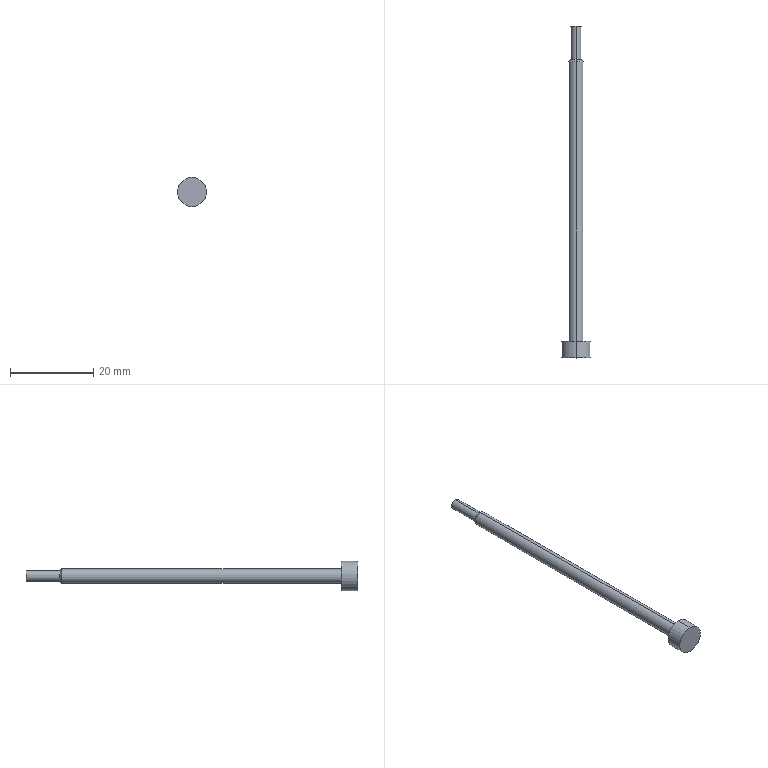Part | STEP file | 1 solid | 11 faces | box 7 x 79.697 x 7 mm | volume 843.527 mm3 | cylinder 6 | plane 3 | cone 2 | commonest cylinder face diameters 2.513 x2 3.5 x2 7 x2
STEP:
#1=CARTESIAN_POINT('',(0.,0.,0.));
#2=DIRECTION('',(0.,0.,1.));
#3=DIRECTION('',(1.,0.,0.));
#4=AXIS2_PLACEMENT_3D('',#1,#2,#3);
#5=CARTESIAN_POINT('',(-37.537,-40.,127.416));
#6=VERTEX_POINT('',#5);
#7=CARTESIAN_POINT('',(-37.537,-40.,120.416));
#8=VERTEX_POINT('',#7);
#9=CARTESIAN_POINT('',(-37.537,-40.,123.916));
#10=DIRECTION('',(0.,1.,0.));
#11=DIRECTION('',(0.,0.,-1.));
#12=AXIS2_PLACEMENT_3D('',#9,#10,#11);
#13=CIRCLE('',#12,3.5);
#14=CARTESIAN_POINT('',(-37.537,-50.,123.916));
#15=DIRECTION('',(0.,1.,0.));
#16=DIRECTION('',(0.,0.,1.));
#17=AXIS2_PLACEMENT_3D('',#14,#15,#16);
#18=CYLINDRICAL_SURFACE('',#17,3.5);
#19=CARTESIAN_POINT('',(-3.142,10.));
#20=DIRECTION('',(1.,0.));
#21=VECTOR('',#20,1.);
#22=LINE('',#19,#21);
#23=(GEOMETRIC_REPRESENTATION_CONTEXT(2)PARAMETRIC_REPRESENTATION_CONTEXT()REPRESENTATION_CONTEXT('',''));
#24=DEFINITIONAL_REPRESENTATION('',(#22),#23);
#25=PCURVE('',#18,#24);
#26=CARTESIAN_POINT('',(-72.862,-40.,23.556));
#27=DIRECTION('',(0.,-1.,0.));
#28=DIRECTION('',(0.,0.,-1.));
#29=AXIS2_PLACEMENT_3D('',#26,#27,#28);
#30=PLANE('',#29);
#31=CARTESIAN_POINT('',(-96.861,35.326));
#32=CARTESIAN_POINT('',(-96.861,29.264));
#33=CARTESIAN_POINT('',(-102.111,32.295));
#34=CARTESIAN_POINT('',(-107.361,35.326));
#35=CARTESIAN_POINT('',(-102.111,38.357));
#36=CARTESIAN_POINT('',(-96.861,41.388));
#37=CARTESIAN_POINT('',(-96.861,35.326));
#38=(BOUNDED_CURVE()B_SPLINE_CURVE(2,(#31,#32,#33,#34,#35,#36,#37),.UNSPECIFIED.,.T.,.F.)B_SPLINE_CURVE_WITH_KNOTS((1,2,2,2,2,1),(-2.094,0.,2.094,4.189,6.283,8.378),.UNSPECIFIED.)CURVE()GEOMETRIC_REPRESENTATION_ITEM()RATIONAL_B_SPLINE_CURVE((1.,0.5,1.,0.5,1.,0.5,1.))REPRESENTATION_ITEM(''));
#39=(GEOMETRIC_REPRESENTATION_CONTEXT(2)PARAMETRIC_REPRESENTATION_CONTEXT()REPRESENTATION_CONTEXT('',''));
#40=DEFINITIONAL_REPRESENTATION('',(#38),#39);
#41=PCURVE('',#30,#40);
#42=SURFACE_CURVE('',#13,(#25,#41),.PCURVE_S1.);
#43=EDGE_CURVE('',#6,#8,#42,.T.);
#44=ORIENTED_EDGE('',*,*,#43,.T.);
#45=CARTESIAN_POINT('',(-37.537,-36.,120.416));
#46=VERTEX_POINT('',#45);
#47=CARTESIAN_POINT('',(-37.537,-50.,120.416));
#48=DIRECTION('',(0.,1.,0.));
#49=VECTOR('',#48,1.);
#50=LINE('',#47,#49);
#51=CARTESIAN_POINT('',(3.142,0.));
#52=DIRECTION('',(0.,1.));
#53=VECTOR('',#52,1.);
#54=LINE('',#51,#53);
#55=(GEOMETRIC_REPRESENTATION_CONTEXT(2)PARAMETRIC_REPRESENTATION_CONTEXT()REPRESENTATION_CONTEXT('',''));
#56=DEFINITIONAL_REPRESENTATION('',(#54),#55);
#57=PCURVE('',#18,#56);
#58=CARTESIAN_POINT('',(-37.537,-50.,123.916));
#59=DIRECTION('',(0.,1.,0.));
#60=DIRECTION('',(0.,0.,1.));
#61=AXIS2_PLACEMENT_3D('',#58,#59,#60);
#62=CYLINDRICAL_SURFACE('',#61,3.5);
#63=CARTESIAN_POINT('',(3.142,0.));
#64=DIRECTION('',(0.,1.));
#65=VECTOR('',#64,1.);
#66=LINE('',#63,#65);
#67=(GEOMETRIC_REPRESENTATION_CONTEXT(2)PARAMETRIC_REPRESENTATION_CONTEXT()REPRESENTATION_CONTEXT('',''));
#68=DEFINITIONAL_REPRESENTATION('',(#66),#67);
#69=PCURVE('',#62,#68);
#70=SURFACE_CURVE('',#50,(#57,#69),.PCURVE_S1.);
#71=EDGE_CURVE('',#8,#46,#70,.T.);
#72=ORIENTED_EDGE('',*,*,#71,.T.);
#73=CARTESIAN_POINT('',(-37.537,-36.,127.416));
#74=VERTEX_POINT('',#73);
#75=CARTESIAN_POINT('',(-37.537,-36.,123.916));
#76=DIRECTION('',(0.,-1.,0.));
#77=DIRECTION('',(0.,0.,-1.));
#78=AXIS2_PLACEMENT_3D('',#75,#76,#77);
#79=CIRCLE('',#78,3.5);
#80=CARTESIAN_POINT('',(3.142,14.));
#81=DIRECTION('',(-1.,0.));
#82=VECTOR('',#81,1.);
#83=LINE('',#80,#82);
#84=(GEOMETRIC_REPRESENTATION_CONTEXT(2)PARAMETRIC_REPRESENTATION_CONTEXT()REPRESENTATION_CONTEXT('',''));
#85=DEFINITIONAL_REPRESENTATION('',(#83),#84);
#86=PCURVE('',#18,#85);
#87=CARTESIAN_POINT('',(-37.537,-36.,123.916));
#88=DIRECTION('',(0.,1.,0.));
#89=DIRECTION('',(0.,0.,1.));
#90=AXIS2_PLACEMENT_3D('',#87,#88,#89);
#91=PLANE('',#90);
#92=CARTESIAN_POINT('',(-3.5,0.));
#93=CARTESIAN_POINT('',(-3.5,6.062));
#94=CARTESIAN_POINT('',(1.75,3.031));
#95=CARTESIAN_POINT('',(7.,0.));
#96=CARTESIAN_POINT('',(1.75,-3.031));
#97=CARTESIAN_POINT('',(-3.5,-6.062));
#98=CARTESIAN_POINT('',(-3.5,0.));
#99=(BOUNDED_CURVE()B_SPLINE_CURVE(2,(#92,#93,#94,#95,#96,#97,#98),.UNSPECIFIED.,.T.,.F.)B_SPLINE_CURVE_WITH_KNOTS((1,2,2,2,2,1),(-2.094,0.,2.094,4.189,6.283,8.378),.UNSPECIFIED.)CURVE()GEOMETRIC_REPRESENTATION_ITEM()RATIONAL_B_SPLINE_CURVE((1.,0.5,1.,0.5,1.,0.5,1.))REPRESENTATION_ITEM(''));
#100=(GEOMETRIC_REPRESENTATION_CONTEXT(2)PARAMETRIC_REPRESENTATION_CONTEXT()REPRESENTATION_CONTEXT('',''));
#101=DEFINITIONAL_REPRESENTATION('',(#99),#100);
#102=PCURVE('',#91,#101);
#103=SURFACE_CURVE('',#79,(#86,#102),.PCURVE_S1.);
#104=EDGE_CURVE('',#46,#74,#103,.T.);
#105=ORIENTED_EDGE('',*,*,#104,.T.);
#106=CARTESIAN_POINT('',(-37.537,-50.,127.416));
#107=DIRECTION('',(0.,1.,0.));
#108=VECTOR('',#107,1.);
#109=LINE('',#106,#108);
#110=CARTESIAN_POINT('',(0.,0.));
#111=DIRECTION('',(0.,1.));
#112=VECTOR('',#111,1.);
#113=LINE('',#110,#112);
#114=(GEOMETRIC_REPRESENTATION_CONTEXT(2)PARAMETRIC_REPRESENTATION_CONTEXT()REPRESENTATION_CONTEXT('',''));
#115=DEFINITIONAL_REPRESENTATION('',(#113),#114);
#116=PCURVE('',#18,#115);
#117=CARTESIAN_POINT('',(6.283,0.));
#118=DIRECTION('',(0.,1.));
#119=VECTOR('',#118,1.);
#120=LINE('',#117,#119);
#121=(GEOMETRIC_REPRESENTATION_CONTEXT(2)PARAMETRIC_REPRESENTATION_CONTEXT()REPRESENTATION_CONTEXT('',''));
#122=DEFINITIONAL_REPRESENTATION('',(#120),#121);
#123=PCURVE('',#62,#122);
#124=SURFACE_CURVE('',#109,(#116,#123),.PCURVE_S1.);
#125=EDGE_CURVE('',#6,#74,#124,.T.);
#126=ORIENTED_EDGE('',*,*,#125,.F.);
#127=EDGE_LOOP('',(#44,#72,#105,#126));
#128=FACE_BOUND('',#127,.T.);
#129=ADVANCED_FACE('',(#128),#18,.T.);
#130=CARTESIAN_POINT('',(-37.537,31.164,125.666));
#131=VERTEX_POINT('',#130);
#132=CARTESIAN_POINT('',(-37.537,31.164,122.166));
#133=VERTEX_POINT('',#132);
#134=CARTESIAN_POINT('',(-37.537,31.164,123.916));
#135=DIRECTION('',(0.,1.,0.));
#136=DIRECTION('',(0.,0.,-1.));
#137=AXIS2_PLACEMENT_3D('',#134,#135,#136);
#138=CIRCLE('',#137,1.75);
#139=CARTESIAN_POINT('',(-37.537,39.697,123.916));
#140=DIRECTION('',(0.,-1.,0.));
#141=DIRECTION('',(0.,0.,-1.));
#142=AXIS2_PLACEMENT_3D('',#139,#140,#141);
#143=CYLINDRICAL_SURFACE('',#142,1.75);
#144=CARTESIAN_POINT('',(6.283,8.534));
#145=DIRECTION('',(-1.,0.));
#146=VECTOR('',#145,1.);
#147=LINE('',#144,#146);
#148=(GEOMETRIC_REPRESENTATION_CONTEXT(2)PARAMETRIC_REPRESENTATION_CONTEXT()REPRESENTATION_CONTEXT('',''));
#149=DEFINITIONAL_REPRESENTATION('',(#147),#148);
#150=PCURVE('',#143,#149);
#151=CARTESIAN_POINT('',(-37.537,31.657,123.916));
#152=DIRECTION('',(0.,-1.,0.));
#153=DIRECTION('',(0.,0.,-1.));
#154=AXIS2_PLACEMENT_3D('',#151,#152,#153);
#155=CONICAL_SURFACE('',#154,1.256,0.7854);
#156=CARTESIAN_POINT('',(6.283,0.4938));
#157=DIRECTION('',(-1.,0.));
#158=VECTOR('',#157,1.);
#159=LINE('',#156,#158);
#160=(GEOMETRIC_REPRESENTATION_CONTEXT(2)PARAMETRIC_REPRESENTATION_CONTEXT()REPRESENTATION_CONTEXT('',''));
#161=DEFINITIONAL_REPRESENTATION('',(#159),#160);
#162=PCURVE('',#155,#161);
#163=SURFACE_CURVE('',#138,(#150,#162),.PCURVE_S1.);
#164=EDGE_CURVE('',#131,#133,#163,.T.);
#165=ORIENTED_EDGE('',*,*,#164,.F.);
#166=CARTESIAN_POINT('',(-37.537,-36.,125.666));
#167=VERTEX_POINT('',#166);
#168=CARTESIAN_POINT('',(-37.537,39.697,125.666));
#169=DIRECTION('',(0.,-1.,0.));
#170=VECTOR('',#169,1.);
#171=LINE('',#168,#170);
#172=CARTESIAN_POINT('',(3.142,0.));
#173=DIRECTION('',(0.,1.));
#174=VECTOR('',#173,1.);
#175=LINE('',#172,#174);
#176=(GEOMETRIC_REPRESENTATION_CONTEXT(2)PARAMETRIC_REPRESENTATION_CONTEXT()REPRESENTATION_CONTEXT('',''));
#177=DEFINITIONAL_REPRESENTATION('',(#175),#176);
#178=PCURVE('',#143,#177);
#179=CARTESIAN_POINT('',(-37.537,39.697,123.916));
#180=DIRECTION('',(0.,-1.,0.));
#181=DIRECTION('',(0.,0.,-1.));
#182=AXIS2_PLACEMENT_3D('',#179,#180,#181);
#183=CYLINDRICAL_SURFACE('',#182,1.75);
#184=CARTESIAN_POINT('',(3.142,0.));
#185=DIRECTION('',(0.,1.));
#186=VECTOR('',#185,1.);
#187=LINE('',#184,#186);
#188=(GEOMETRIC_REPRESENTATION_CONTEXT(2)PARAMETRIC_REPRESENTATION_CONTEXT()REPRESENTATION_CONTEXT('',''));
#189=DEFINITIONAL_REPRESENTATION('',(#187),#188);
#190=PCURVE('',#183,#189);
#191=SURFACE_CURVE('',#171,(#178,#190),.PCURVE_S1.);
#192=EDGE_CURVE('',#131,#167,#191,.T.);
#193=ORIENTED_EDGE('',*,*,#192,.T.);
#194=CARTESIAN_POINT('',(-37.537,-36.,122.166));
#195=VERTEX_POINT('',#194);
#196=CARTESIAN_POINT('',(-37.537,-36.,123.916));
#197=DIRECTION('',(0.,-1.,0.));
#198=DIRECTION('',(0.,0.,1.));
#199=AXIS2_PLACEMENT_3D('',#196,#197,#198);
#200=CIRCLE('',#199,1.75);
#201=CARTESIAN_POINT('',(-3.142,75.698));
#202=DIRECTION('',(1.,0.));
#203=VECTOR('',#202,1.);
#204=LINE('',#201,#203);
#205=(GEOMETRIC_REPRESENTATION_CONTEXT(2)PARAMETRIC_REPRESENTATION_CONTEXT()REPRESENTATION_CONTEXT('',''));
#206=DEFINITIONAL_REPRESENTATION('',(#204),#205);
#207=PCURVE('',#143,#206);
#208=CARTESIAN_POINT('',(1.75,0.));
#209=CARTESIAN_POINT('',(1.75,-3.031));
#210=CARTESIAN_POINT('',(-0.875,-1.516));
#211=CARTESIAN_POINT('',(-3.5,0.));
#212=CARTESIAN_POINT('',(-0.875,1.516));
#213=CARTESIAN_POINT('',(1.75,3.031));
#214=CARTESIAN_POINT('',(1.75,0.));
#215=(BOUNDED_CURVE()B_SPLINE_CURVE(2,(#208,#209,#210,#211,#212,#213,#214),.UNSPECIFIED.,.T.,.F.)B_SPLINE_CURVE_WITH_KNOTS((1,2,2,2,2,1),(-2.094,0.,2.094,4.189,6.283,8.378),.UNSPECIFIED.)CURVE()GEOMETRIC_REPRESENTATION_ITEM()RATIONAL_B_SPLINE_CURVE((1.,0.5,1.,0.5,1.,0.5,1.))REPRESENTATION_ITEM(''));
#216=(GEOMETRIC_REPRESENTATION_CONTEXT(2)PARAMETRIC_REPRESENTATION_CONTEXT()REPRESENTATION_CONTEXT('',''));
#217=DEFINITIONAL_REPRESENTATION('',(#215),#216);
#218=PCURVE('',#91,#217);
#219=SURFACE_CURVE('',#200,(#207,#218),.PCURVE_S1.);
#220=EDGE_CURVE('',#195,#167,#219,.T.);
#221=ORIENTED_EDGE('',*,*,#220,.F.);
#222=CARTESIAN_POINT('',(-37.537,39.697,122.166));
#223=DIRECTION('',(0.,-1.,0.));
#224=VECTOR('',#223,1.);
#225=LINE('',#222,#224);
#226=CARTESIAN_POINT('',(0.,0.));
#227=DIRECTION('',(0.,1.));
#228=VECTOR('',#227,1.);
#229=LINE('',#226,#228);
#230=(GEOMETRIC_REPRESENTATION_CONTEXT(2)PARAMETRIC_REPRESENTATION_CONTEXT()REPRESENTATION_CONTEXT('',''));
#231=DEFINITIONAL_REPRESENTATION('',(#229),#230);
#232=PCURVE('',#143,#231);
#233=CARTESIAN_POINT('',(6.283,0.));
#234=DIRECTION('',(0.,1.));
#235=VECTOR('',#234,1.);
#236=LINE('',#233,#235);
#237=(GEOMETRIC_REPRESENTATION_CONTEXT(2)PARAMETRIC_REPRESENTATION_CONTEXT()REPRESENTATION_CONTEXT('',''));
#238=DEFINITIONAL_REPRESENTATION('',(#236),#237);
#239=PCURVE('',#183,#238);
#240=SURFACE_CURVE('',#225,(#232,#239),.PCURVE_S1.);
#241=EDGE_CURVE('',#133,#195,#240,.T.);
#242=ORIENTED_EDGE('',*,*,#241,.F.);
#243=EDGE_LOOP('',(#165,#193,#221,#242));
#244=FACE_BOUND('',#243,.T.);
#245=ADVANCED_FACE('',(#244),#143,.T.);
#246=CARTESIAN_POINT('',(-37.537,31.657,122.66));
#247=VERTEX_POINT('',#246);
#248=CARTESIAN_POINT('',(-37.537,31.657,125.173));
#249=VERTEX_POINT('',#248);
#250=CARTESIAN_POINT('',(-37.537,31.657,123.916));
#251=DIRECTION('',(0.,-1.,0.));
#252=DIRECTION('',(0.,0.,-1.));
#253=AXIS2_PLACEMENT_3D('',#250,#251,#252);
#254=CIRCLE('',#253,1.256);
#255=CARTESIAN_POINT('',(0.,0.));
#256=DIRECTION('',(1.,0.));
#257=VECTOR('',#256,1.);
#258=LINE('',#255,#257);
#259=(GEOMETRIC_REPRESENTATION_CONTEXT(2)PARAMETRIC_REPRESENTATION_CONTEXT()REPRESENTATION_CONTEXT('',''));
#260=DEFINITIONAL_REPRESENTATION('',(#258),#259);
#261=PCURVE('',#155,#260);
#262=CARTESIAN_POINT('',(-37.537,39.697,123.916));
#263=DIRECTION('',(0.,-1.,0.));
#264=DIRECTION('',(0.,0.,-1.));
#265=AXIS2_PLACEMENT_3D('',#262,#263,#264);
#266=CYLINDRICAL_SURFACE('',#265,1.256);
#267=CARTESIAN_POINT('',(0.,8.04));
#268=DIRECTION('',(1.,0.));
#269=VECTOR('',#268,1.);
#270=LINE('',#267,#269);
#271=(GEOMETRIC_REPRESENTATION_CONTEXT(2)PARAMETRIC_REPRESENTATION_CONTEXT()REPRESENTATION_CONTEXT('',''));
#272=DEFINITIONAL_REPRESENTATION('',(#270),#271);
#273=PCURVE('',#266,#272);
#274=SURFACE_CURVE('',#254,(#261,#273),.PCURVE_S1.);
#275=EDGE_CURVE('',#247,#249,#274,.T.);
#276=ORIENTED_EDGE('',*,*,#275,.T.);
#277=CARTESIAN_POINT('',(-37.537,31.657,125.173));
#278=DIRECTION('',(0.,-0.7071,0.7071));
#279=VECTOR('',#278,1.);
#280=LINE('',#277,#279);
#281=CARTESIAN_POINT('',(3.142,0.));
#282=DIRECTION('',(0.,1.));
#283=VECTOR('',#282,1.);
#284=LINE('',#281,#283);
#285=(GEOMETRIC_REPRESENTATION_CONTEXT(2)PARAMETRIC_REPRESENTATION_CONTEXT()REPRESENTATION_CONTEXT('',''));
#286=DEFINITIONAL_REPRESENTATION('',(#284),#285);
#287=PCURVE('',#155,#286);
#288=CARTESIAN_POINT('',(-37.537,31.657,123.916));
#289=DIRECTION('',(0.,-1.,0.));
#290=DIRECTION('',(0.,0.,-1.));
#291=AXIS2_PLACEMENT_3D('',#288,#289,#290);
#292=CONICAL_SURFACE('',#291,1.256,0.7854);
#293=CARTESIAN_POINT('',(3.142,0.));
#294=DIRECTION('',(0.,1.));
#295=VECTOR('',#294,1.);
#296=LINE('',#293,#295);
#297=(GEOMETRIC_REPRESENTATION_CONTEXT(2)PARAMETRIC_REPRESENTATION_CONTEXT()REPRESENTATION_CONTEXT('',''));
#298=DEFINITIONAL_REPRESENTATION('',(#296),#297);
#299=PCURVE('',#292,#298);
#300=SURFACE_CURVE('',#280,(#287,#299),.PCURVE_S1.);
#301=EDGE_CURVE('',#249,#131,#300,.T.);
#302=ORIENTED_EDGE('',*,*,#301,.T.);
#303=ORIENTED_EDGE('',*,*,#164,.T.);
#304=CARTESIAN_POINT('',(-37.537,31.657,122.66));
#305=DIRECTION('',(0.,-0.7071,-0.7071));
#306=VECTOR('',#305,1.);
#307=LINE('',#304,#306);
#308=CARTESIAN_POINT('',(0.,0.));
#309=DIRECTION('',(0.,1.));
#310=VECTOR('',#309,1.);
#311=LINE('',#308,#310);
#312=(GEOMETRIC_REPRESENTATION_CONTEXT(2)PARAMETRIC_REPRESENTATION_CONTEXT()REPRESENTATION_CONTEXT('',''));
#313=DEFINITIONAL_REPRESENTATION('',(#311),#312);
#314=PCURVE('',#155,#313);
#315=CARTESIAN_POINT('',(6.283,0.));
#316=DIRECTION('',(0.,1.));
#317=VECTOR('',#316,1.);
#318=LINE('',#315,#317);
#319=(GEOMETRIC_REPRESENTATION_CONTEXT(2)PARAMETRIC_REPRESENTATION_CONTEXT()REPRESENTATION_CONTEXT('',''));
#320=DEFINITIONAL_REPRESENTATION('',(#318),#319);
#321=PCURVE('',#292,#320);
#322=SURFACE_CURVE('',#307,(#314,#321),.PCURVE_S1.);
#323=EDGE_CURVE('',#247,#133,#322,.T.);
#324=ORIENTED_EDGE('',*,*,#323,.F.);
#325=EDGE_LOOP('',(#276,#302,#303,#324));
#326=FACE_BOUND('',#325,.T.);
#327=ADVANCED_FACE('',(#326),#155,.T.);
#328=CARTESIAN_POINT('',(-37.537,39.697,122.66));
#329=VERTEX_POINT('',#328);
#330=CARTESIAN_POINT('',(-37.537,39.697,125.173));
#331=VERTEX_POINT('',#330);
#332=CARTESIAN_POINT('',(-37.537,39.697,123.916));
#333=DIRECTION('',(0.,-1.,0.));
#334=DIRECTION('',(0.,0.,-1.));
#335=AXIS2_PLACEMENT_3D('',#332,#333,#334);
#336=CIRCLE('',#335,1.256);
#337=CARTESIAN_POINT('',(0.,0.));
#338=DIRECTION('',(1.,0.));
#339=VECTOR('',#338,1.);
#340=LINE('',#337,#339);
#341=(GEOMETRIC_REPRESENTATION_CONTEXT(2)PARAMETRIC_REPRESENTATION_CONTEXT()REPRESENTATION_CONTEXT('',''));
#342=DEFINITIONAL_REPRESENTATION('',(#340),#341);
#343=PCURVE('',#266,#342);
#344=CARTESIAN_POINT('',(-37.537,39.697,123.916));
#345=DIRECTION('',(0.,1.,0.));
#346=DIRECTION('',(0.,0.,1.));
#347=AXIS2_PLACEMENT_3D('',#344,#345,#346);
#348=PLANE('',#347);
#349=CARTESIAN_POINT('',(-1.256,0.));
#350=CARTESIAN_POINT('',(-1.256,2.176));
#351=CARTESIAN_POINT('',(0.6281,1.088));
#352=CARTESIAN_POINT('',(2.513,0.));
#353=CARTESIAN_POINT('',(0.6281,-1.088));
#354=CARTESIAN_POINT('',(-1.256,-2.176));
#355=CARTESIAN_POINT('',(-1.256,0.));
#356=(BOUNDED_CURVE()B_SPLINE_CURVE(2,(#349,#350,#351,#352,#353,#354,#355),.UNSPECIFIED.,.T.,.F.)B_SPLINE_CURVE_WITH_KNOTS((1,2,2,2,2,1),(-2.094,0.,2.094,4.189,6.283,8.378),.UNSPECIFIED.)CURVE()GEOMETRIC_REPRESENTATION_ITEM()RATIONAL_B_SPLINE_CURVE((1.,0.5,1.,0.5,1.,0.5,1.))REPRESENTATION_ITEM(''));
#357=(GEOMETRIC_REPRESENTATION_CONTEXT(2)PARAMETRIC_REPRESENTATION_CONTEXT()REPRESENTATION_CONTEXT('',''));
#358=DEFINITIONAL_REPRESENTATION('',(#356),#357);
#359=PCURVE('',#348,#358);
#360=SURFACE_CURVE('',#336,(#343,#359),.PCURVE_S1.);
#361=EDGE_CURVE('',#329,#331,#360,.T.);
#362=ORIENTED_EDGE('',*,*,#361,.T.);
#363=CARTESIAN_POINT('',(-37.537,39.697,125.173));
#364=DIRECTION('',(0.,-1.,0.));
#365=VECTOR('',#364,1.);
#366=LINE('',#363,#365);
#367=CARTESIAN_POINT('',(3.142,0.));
#368=DIRECTION('',(0.,1.));
#369=VECTOR('',#368,1.);
#370=LINE('',#367,#369);
#371=(GEOMETRIC_REPRESENTATION_CONTEXT(2)PARAMETRIC_REPRESENTATION_CONTEXT()REPRESENTATION_CONTEXT('',''));
#372=DEFINITIONAL_REPRESENTATION('',(#370),#371);
#373=PCURVE('',#266,#372);
#374=CARTESIAN_POINT('',(-37.537,39.697,123.916));
#375=DIRECTION('',(0.,-1.,0.));
#376=DIRECTION('',(0.,0.,-1.));
#377=AXIS2_PLACEMENT_3D('',#374,#375,#376);
#378=CYLINDRICAL_SURFACE('',#377,1.256);
#379=CARTESIAN_POINT('',(3.142,0.));
#380=DIRECTION('',(0.,1.));
#381=VECTOR('',#380,1.);
#382=LINE('',#379,#381);
#383=(GEOMETRIC_REPRESENTATION_CONTEXT(2)PARAMETRIC_REPRESENTATION_CONTEXT()REPRESENTATION_CONTEXT('',''));
#384=DEFINITIONAL_REPRESENTATION('',(#382),#383);
#385=PCURVE('',#378,#384);
#386=SURFACE_CURVE('',#366,(#373,#385),.PCURVE_S1.);
#387=EDGE_CURVE('',#331,#249,#386,.T.);
#388=ORIENTED_EDGE('',*,*,#387,.T.);
#389=ORIENTED_EDGE('',*,*,#275,.F.);
#390=CARTESIAN_POINT('',(-37.537,39.697,122.66));
#391=DIRECTION('',(0.,-1.,0.));
#392=VECTOR('',#391,1.);
#393=LINE('',#390,#392);
#394=CARTESIAN_POINT('',(0.,0.));
#395=DIRECTION('',(0.,1.));
#396=VECTOR('',#395,1.);
#397=LINE('',#394,#396);
#398=(GEOMETRIC_REPRESENTATION_CONTEXT(2)PARAMETRIC_REPRESENTATION_CONTEXT()REPRESENTATION_CONTEXT('',''));
#399=DEFINITIONAL_REPRESENTATION('',(#397),#398);
#400=PCURVE('',#266,#399);
#401=CARTESIAN_POINT('',(6.283,0.));
#402=DIRECTION('',(0.,1.));
#403=VECTOR('',#402,1.);
#404=LINE('',#401,#403);
#405=(GEOMETRIC_REPRESENTATION_CONTEXT(2)PARAMETRIC_REPRESENTATION_CONTEXT()REPRESENTATION_CONTEXT('',''));
#406=DEFINITIONAL_REPRESENTATION('',(#404),#405);
#407=PCURVE('',#378,#406);
#408=SURFACE_CURVE('',#393,(#400,#407),.PCURVE_S1.);
#409=EDGE_CURVE('',#329,#247,#408,.T.);
#410=ORIENTED_EDGE('',*,*,#409,.F.);
#411=EDGE_LOOP('',(#362,#388,#389,#410));
#412=FACE_BOUND('',#411,.T.);
#413=ADVANCED_FACE('',(#412),#266,.T.);
#414=ORIENTED_EDGE('',*,*,#387,.F.);
#415=CARTESIAN_POINT('',(-37.537,39.697,123.916));
#416=DIRECTION('',(0.,-1.,0.));
#417=DIRECTION('',(0.,0.,-1.));
#418=AXIS2_PLACEMENT_3D('',#415,#416,#417);
#419=CIRCLE('',#418,1.256);
#420=CARTESIAN_POINT('',(0.,0.));
#421=DIRECTION('',(1.,0.));
#422=VECTOR('',#421,1.);
#423=LINE('',#420,#422);
#424=(GEOMETRIC_REPRESENTATION_CONTEXT(2)PARAMETRIC_REPRESENTATION_CONTEXT()REPRESENTATION_CONTEXT('',''));
#425=DEFINITIONAL_REPRESENTATION('',(#423),#424);
#426=PCURVE('',#378,#425);
#427=CARTESIAN_POINT('',(-1.256,0.));
#428=CARTESIAN_POINT('',(-1.256,2.176));
#429=CARTESIAN_POINT('',(0.6281,1.088));
#430=CARTESIAN_POINT('',(2.513,0.));
#431=CARTESIAN_POINT('',(0.6281,-1.088));
#432=CARTESIAN_POINT('',(-1.256,-2.176));
#433=CARTESIAN_POINT('',(-1.256,0.));
#434=(BOUNDED_CURVE()B_SPLINE_CURVE(2,(#427,#428,#429,#430,#431,#432,#433),.UNSPECIFIED.,.T.,.F.)B_SPLINE_CURVE_WITH_KNOTS((1,2,2,2,2,1),(-2.094,0.,2.094,4.189,6.283,8.378),.UNSPECIFIED.)CURVE()GEOMETRIC_REPRESENTATION_ITEM()RATIONAL_B_SPLINE_CURVE((1.,0.5,1.,0.5,1.,0.5,1.))REPRESENTATION_ITEM(''));
#435=(GEOMETRIC_REPRESENTATION_CONTEXT(2)PARAMETRIC_REPRESENTATION_CONTEXT()REPRESENTATION_CONTEXT('',''));
#436=DEFINITIONAL_REPRESENTATION('',(#434),#435);
#437=PCURVE('',#348,#436);
#438=SURFACE_CURVE('',#419,(#426,#437),.PCURVE_S1.);
#439=EDGE_CURVE('',#331,#329,#438,.T.);
#440=ORIENTED_EDGE('',*,*,#439,.T.);
#441=ORIENTED_EDGE('',*,*,#409,.T.);
#442=CARTESIAN_POINT('',(-37.537,31.657,123.916));
#443=DIRECTION('',(0.,-1.,0.));
#444=DIRECTION('',(0.,0.,-1.));
#445=AXIS2_PLACEMENT_3D('',#442,#443,#444);
#446=CIRCLE('',#445,1.256);
#447=CARTESIAN_POINT('',(0.,8.04));
#448=DIRECTION('',(1.,0.));
#449=VECTOR('',#448,1.);
#450=LINE('',#447,#449);
#451=(GEOMETRIC_REPRESENTATION_CONTEXT(2)PARAMETRIC_REPRESENTATION_CONTEXT()REPRESENTATION_CONTEXT('',''));
#452=DEFINITIONAL_REPRESENTATION('',(#450),#451);
#453=PCURVE('',#378,#452);
#454=CARTESIAN_POINT('',(0.,0.));
#455=DIRECTION('',(1.,0.));
#456=VECTOR('',#455,1.);
#457=LINE('',#454,#456);
#458=(GEOMETRIC_REPRESENTATION_CONTEXT(2)PARAMETRIC_REPRESENTATION_CONTEXT()REPRESENTATION_CONTEXT('',''));
#459=DEFINITIONAL_REPRESENTATION('',(#457),#458);
#460=PCURVE('',#292,#459);
#461=SURFACE_CURVE('',#446,(#453,#460),.PCURVE_S1.);
#462=EDGE_CURVE('',#249,#247,#461,.T.);
#463=ORIENTED_EDGE('',*,*,#462,.F.);
#464=EDGE_LOOP('',(#414,#440,#441,#463));
#465=FACE_BOUND('',#464,.T.);
#466=ADVANCED_FACE('',(#465),#378,.T.);
#467=ORIENTED_EDGE('',*,*,#301,.F.);
#468=ORIENTED_EDGE('',*,*,#462,.T.);
#469=ORIENTED_EDGE('',*,*,#323,.T.);
#470=CARTESIAN_POINT('',(-37.537,31.164,123.916));
#471=DIRECTION('',(0.,1.,0.));
#472=DIRECTION('',(0.,0.,-1.));
#473=AXIS2_PLACEMENT_3D('',#470,#471,#472);
#474=CIRCLE('',#473,1.75);
#475=CARTESIAN_POINT('',(6.283,0.4938));
#476=DIRECTION('',(-1.,0.));
#477=VECTOR('',#476,1.);
#478=LINE('',#475,#477);
#479=(GEOMETRIC_REPRESENTATION_CONTEXT(2)PARAMETRIC_REPRESENTATION_CONTEXT()REPRESENTATION_CONTEXT('',''));
#480=DEFINITIONAL_REPRESENTATION('',(#478),#479);
#481=PCURVE('',#292,#480);
#482=CARTESIAN_POINT('',(6.283,8.534));
#483=DIRECTION('',(-1.,0.));
#484=VECTOR('',#483,1.);
#485=LINE('',#482,#484);
#486=(GEOMETRIC_REPRESENTATION_CONTEXT(2)PARAMETRIC_REPRESENTATION_CONTEXT()REPRESENTATION_CONTEXT('',''));
#487=DEFINITIONAL_REPRESENTATION('',(#485),#486);
#488=PCURVE('',#183,#487);
#489=SURFACE_CURVE('',#474,(#481,#488),.PCURVE_S1.);
#490=EDGE_CURVE('',#133,#131,#489,.T.);
#491=ORIENTED_EDGE('',*,*,#490,.T.);
#492=EDGE_LOOP('',(#467,#468,#469,#491));
#493=FACE_BOUND('',#492,.T.);
#494=ADVANCED_FACE('',(#493),#292,.T.);
#495=ORIENTED_EDGE('',*,*,#192,.F.);
#496=ORIENTED_EDGE('',*,*,#490,.F.);
#497=ORIENTED_EDGE('',*,*,#241,.T.);
#498=CARTESIAN_POINT('',(-37.537,-36.,123.916));
#499=DIRECTION('',(0.,-1.,0.));
#500=DIRECTION('',(0.,0.,1.));
#501=AXIS2_PLACEMENT_3D('',#498,#499,#500);
#502=CIRCLE('',#501,1.75);
#503=CARTESIAN_POINT('',(3.142,75.698));
#504=DIRECTION('',(1.,0.));
#505=VECTOR('',#504,1.);
#506=LINE('',#503,#505);
#507=(GEOMETRIC_REPRESENTATION_CONTEXT(2)PARAMETRIC_REPRESENTATION_CONTEXT()REPRESENTATION_CONTEXT('',''));
#508=DEFINITIONAL_REPRESENTATION('',(#506),#507);
#509=PCURVE('',#183,#508);
#510=CARTESIAN_POINT('',(1.75,0.));
#511=CARTESIAN_POINT('',(1.75,-3.031));
#512=CARTESIAN_POINT('',(-0.875,-1.516));
#513=CARTESIAN_POINT('',(-3.5,0.));
#514=CARTESIAN_POINT('',(-0.875,1.516));
#515=CARTESIAN_POINT('',(1.75,3.031));
#516=CARTESIAN_POINT('',(1.75,0.));
#517=(BOUNDED_CURVE()B_SPLINE_CURVE(2,(#510,#511,#512,#513,#514,#515,#516),.UNSPECIFIED.,.T.,.F.)B_SPLINE_CURVE_WITH_KNOTS((1,2,2,2,2,1),(-2.094,0.,2.094,4.189,6.283,8.378),.UNSPECIFIED.)CURVE()GEOMETRIC_REPRESENTATION_ITEM()RATIONAL_B_SPLINE_CURVE((1.,0.5,1.,0.5,1.,0.5,1.))REPRESENTATION_ITEM(''));
#518=(GEOMETRIC_REPRESENTATION_CONTEXT(2)PARAMETRIC_REPRESENTATION_CONTEXT()REPRESENTATION_CONTEXT('',''));
#519=DEFINITIONAL_REPRESENTATION('',(#517),#518);
#520=PCURVE('',#91,#519);
#521=SURFACE_CURVE('',#502,(#509,#520),.PCURVE_S1.);
#522=EDGE_CURVE('',#167,#195,#521,.T.);
#523=ORIENTED_EDGE('',*,*,#522,.F.);
#524=EDGE_LOOP('',(#495,#496,#497,#523));
#525=FACE_BOUND('',#524,.T.);
#526=ADVANCED_FACE('',(#525),#183,.T.);
#527=ORIENTED_EDGE('',*,*,#361,.F.);
#528=ORIENTED_EDGE('',*,*,#439,.F.);
#529=EDGE_LOOP('',(#527,#528));
#530=FACE_BOUND('',#529,.T.);
#531=ADVANCED_FACE('',(#530),#348,.T.);
#532=ORIENTED_EDGE('',*,*,#220,.T.);
#533=ORIENTED_EDGE('',*,*,#522,.T.);
#534=EDGE_LOOP('',(#532,#533));
#535=FACE_BOUND('',#534,.T.);
#536=CARTESIAN_POINT('',(-37.537,-36.,123.916));
#537=DIRECTION('',(0.,-1.,0.));
#538=DIRECTION('',(0.,0.,-1.));
#539=AXIS2_PLACEMENT_3D('',#536,#537,#538);
#540=CIRCLE('',#539,3.5);
#541=CARTESIAN_POINT('',(-3.5,0.));
#542=CARTESIAN_POINT('',(-3.5,6.062));
#543=CARTESIAN_POINT('',(1.75,3.031));
#544=CARTESIAN_POINT('',(7.,0.));
#545=CARTESIAN_POINT('',(1.75,-3.031));
#546=CARTESIAN_POINT('',(-3.5,-6.062));
#547=CARTESIAN_POINT('',(-3.5,0.));
#548=(BOUNDED_CURVE()B_SPLINE_CURVE(2,(#541,#542,#543,#544,#545,#546,#547),.UNSPECIFIED.,.T.,.F.)B_SPLINE_CURVE_WITH_KNOTS((1,2,2,2,2,1),(-2.094,0.,2.094,4.189,6.283,8.378),.UNSPECIFIED.)CURVE()GEOMETRIC_REPRESENTATION_ITEM()RATIONAL_B_SPLINE_CURVE((1.,0.5,1.,0.5,1.,0.5,1.))REPRESENTATION_ITEM(''));
#549=(GEOMETRIC_REPRESENTATION_CONTEXT(2)PARAMETRIC_REPRESENTATION_CONTEXT()REPRESENTATION_CONTEXT('',''));
#550=DEFINITIONAL_REPRESENTATION('',(#548),#549);
#551=PCURVE('',#91,#550);
#552=CARTESIAN_POINT('',(9.425,14.));
#553=DIRECTION('',(-1.,0.));
#554=VECTOR('',#553,1.);
#555=LINE('',#552,#554);
#556=(GEOMETRIC_REPRESENTATION_CONTEXT(2)PARAMETRIC_REPRESENTATION_CONTEXT()REPRESENTATION_CONTEXT('',''));
#557=DEFINITIONAL_REPRESENTATION('',(#555),#556);
#558=PCURVE('',#62,#557);
#559=SURFACE_CURVE('',#540,(#551,#558),.PCURVE_S1.);
#560=EDGE_CURVE('',#74,#46,#559,.T.);
#561=ORIENTED_EDGE('',*,*,#560,.F.);
#562=ORIENTED_EDGE('',*,*,#104,.F.);
#563=EDGE_LOOP('',(#561,#562));
#564=FACE_BOUND('',#563,.T.);
#565=ADVANCED_FACE('',(#535,#564),#91,.T.);
#566=ORIENTED_EDGE('',*,*,#71,.F.);
#567=CARTESIAN_POINT('',(-37.537,-40.,123.916));
#568=DIRECTION('',(0.,1.,0.));
#569=DIRECTION('',(0.,0.,-1.));
#570=AXIS2_PLACEMENT_3D('',#567,#568,#569);
#571=CIRCLE('',#570,3.5);
#572=CARTESIAN_POINT('',(3.142,10.));
#573=DIRECTION('',(1.,0.));
#574=VECTOR('',#573,1.);
#575=LINE('',#572,#574);
#576=(GEOMETRIC_REPRESENTATION_CONTEXT(2)PARAMETRIC_REPRESENTATION_CONTEXT()REPRESENTATION_CONTEXT('',''));
#577=DEFINITIONAL_REPRESENTATION('',(#575),#576);
#578=PCURVE('',#62,#577);
#579=CARTESIAN_POINT('',(-96.861,35.326));
#580=CARTESIAN_POINT('',(-96.861,29.264));
#581=CARTESIAN_POINT('',(-102.111,32.295));
#582=CARTESIAN_POINT('',(-107.361,35.326));
#583=CARTESIAN_POINT('',(-102.111,38.357));
#584=CARTESIAN_POINT('',(-96.861,41.388));
#585=CARTESIAN_POINT('',(-96.861,35.326));
#586=(BOUNDED_CURVE()B_SPLINE_CURVE(2,(#579,#580,#581,#582,#583,#584,#585),.UNSPECIFIED.,.T.,.F.)B_SPLINE_CURVE_WITH_KNOTS((1,2,2,2,2,1),(-2.094,0.,2.094,4.189,6.283,8.378),.UNSPECIFIED.)CURVE()GEOMETRIC_REPRESENTATION_ITEM()RATIONAL_B_SPLINE_CURVE((1.,0.5,1.,0.5,1.,0.5,1.))REPRESENTATION_ITEM(''));
#587=(GEOMETRIC_REPRESENTATION_CONTEXT(2)PARAMETRIC_REPRESENTATION_CONTEXT()REPRESENTATION_CONTEXT('',''));
#588=DEFINITIONAL_REPRESENTATION('',(#586),#587);
#589=PCURVE('',#30,#588);
#590=SURFACE_CURVE('',#571,(#578,#589),.PCURVE_S1.);
#591=EDGE_CURVE('',#8,#6,#590,.T.);
#592=ORIENTED_EDGE('',*,*,#591,.T.);
#593=ORIENTED_EDGE('',*,*,#125,.T.);
#594=ORIENTED_EDGE('',*,*,#560,.T.);
#595=EDGE_LOOP('',(#566,#592,#593,#594));
#596=FACE_BOUND('',#595,.T.);
#597=ADVANCED_FACE('',(#596),#62,.T.);
#598=ORIENTED_EDGE('',*,*,#43,.F.);
#599=ORIENTED_EDGE('',*,*,#591,.F.);
#600=EDGE_LOOP('',(#598,#599));
#601=FACE_BOUND('',#600,.T.);
#602=ADVANCED_FACE('',(#601),#30,.T.);
#603=CLOSED_SHELL('',(#129,#245,#327,#413,#466,#494,#526,#531,#565,#597,#602));
#604=MANIFOLD_SOLID_BREP('',#603);
#605=(LENGTH_UNIT()NAMED_UNIT(*)SI_UNIT(.MILLI.,.METRE.));
#606=UNCERTAINTY_MEASURE_WITH_UNIT(LENGTH_MEASURE(0.0000001),#605,'','');
#607=(NAMED_UNIT(*)PLANE_ANGLE_UNIT()SI_UNIT($,.RADIAN.));
#608=(NAMED_UNIT(*)SI_UNIT($,.STERADIAN.)SOLID_ANGLE_UNIT());
#609=(GEOMETRIC_REPRESENTATION_CONTEXT(3)GLOBAL_UNCERTAINTY_ASSIGNED_CONTEXT((#606))GLOBAL_UNIT_ASSIGNED_CONTEXT((#605,#607,#608))REPRESENTATION_CONTEXT('',''));
#610=ADVANCED_BREP_SHAPE_REPRESENTATION('',(#4,#604),#609);